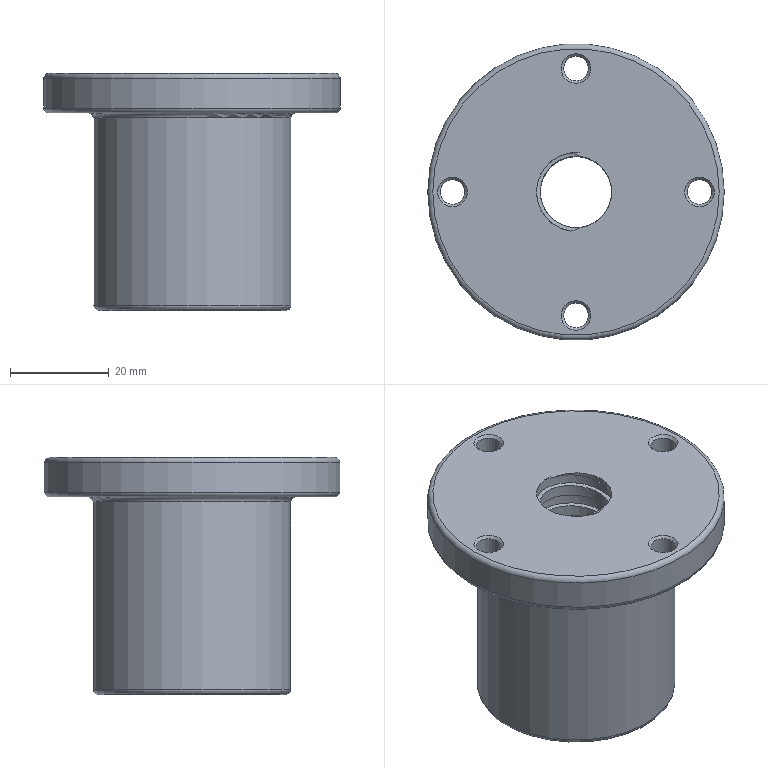Part | NX | features DATUM_CSYS 5, SIMPLE HOLE 4, SKETCH 4, SYMBOLIC_THREAD 4, EXTRUDE 3, BLEND 2, HOLE PACKAGE 1, THREADS 1 | 1 solid | 35 faces | box 60 x 60 x 48 mm | volume 63352 mm3 | cylinder 17 | cone 8 | plane 4 | torus 4 | spline 2 | commonest cylinder face diameters 14.5 x10 5 x4 16 x1 40 x1 60 x1